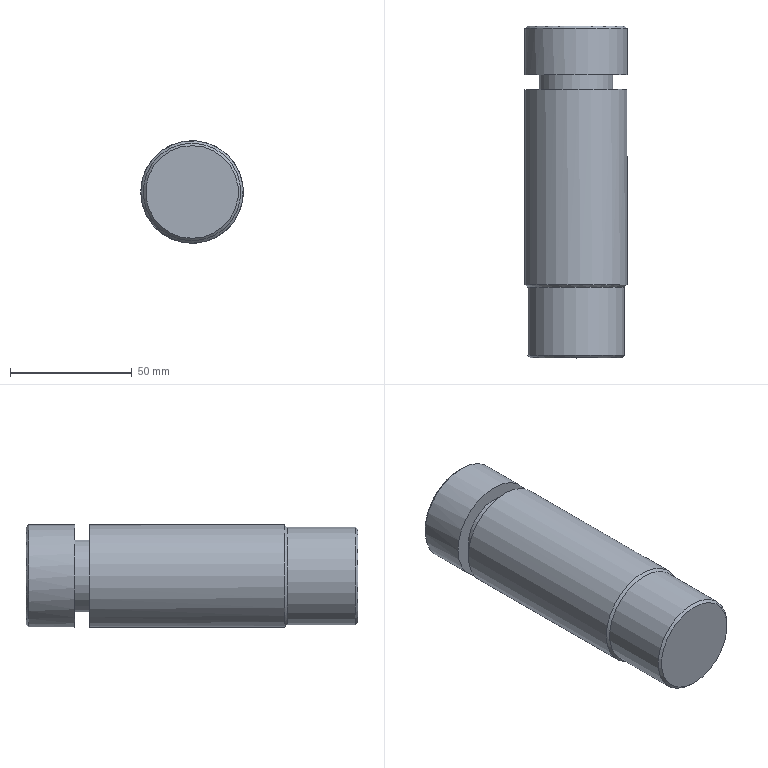Part | NX | features solid 2 | 1 solid | 11 faces | box 42 x 136 x 42 mm | volume 180422 mm3 | plane 4 | cylinder 4 | cone 3 | commonest cylinder face diameters 42 x2 30 x1 40 x1
STEP:
#1=CARTESIAN_POINT('',(1024.,425.,180.));
#2=VERTEX_POINT('',#1);
#3=CARTESIAN_POINT('',(1045.,425.,180.));
#4=DIRECTION('',(0.,1.,0.));
#5=DIRECTION('',(-1.,0.,0.));
#6=AXIS2_PLACEMENT_3D('',#3,#4,#5);
#7=CIRCLE('',#6,21.);
#8=EDGE_CURVE('',#2,#2,#7,.T.);
#9=ORIENTED_EDGE('',*,*,#8,.T.);
#10=EDGE_LOOP('',(#9));
#11=FACE_BOUND('',#10,.T.);
#12=CARTESIAN_POINT('',(1030.,425.,180.));
#13=VERTEX_POINT('',#12);
#14=CARTESIAN_POINT('',(1045.,425.,180.));
#15=DIRECTION('',(0.,1.,0.));
#16=DIRECTION('',(-1.,0.,0.));
#17=AXIS2_PLACEMENT_3D('',#14,#15,#16);
#18=CIRCLE('',#17,15.);
#19=EDGE_CURVE('',#13,#13,#18,.T.);
#20=ORIENTED_EDGE('',*,*,#19,.F.);
#21=EDGE_LOOP('',(#20));
#22=FACE_BOUND('',#21,.T.);
#23=CARTESIAN_POINT('',(1045.,425.,180.));
#24=DIRECTION('',(0.,1.,0.));
#25=DIRECTION('',(0.,0.,-1.));
#26=AXIS2_PLACEMENT_3D('',#23,#24,#25);
#27=PLANE('',#26);
#28=ADVANCED_FACE('',(#11,#22),#27,.T.);
#29=CARTESIAN_POINT('',(1024.,345.,180.));
#30=VERTEX_POINT('',#29);
#31=CARTESIAN_POINT('',(1045.,345.,180.));
#32=DIRECTION('',(0.,1.,0.));
#33=DIRECTION('',(-1.,0.,0.));
#34=AXIS2_PLACEMENT_3D('',#31,#32,#33);
#35=CIRCLE('',#34,21.);
#36=EDGE_CURVE('',#30,#30,#35,.T.);
#37=ORIENTED_EDGE('',*,*,#36,.T.);
#38=EDGE_LOOP('',(#37));
#39=FACE_BOUND('',#38,.T.);
#40=ORIENTED_EDGE('',*,*,#8,.F.);
#41=EDGE_LOOP('',(#40));
#42=FACE_BOUND('',#41,.T.);
#43=CARTESIAN_POINT('',(1045.,405.,180.));
#44=DIRECTION('',(0.,-1.,0.));
#45=DIRECTION('',(0.,0.,1.));
#46=AXIS2_PLACEMENT_3D('',#43,#44,#45);
#47=CYLINDRICAL_SURFACE('',#46,21.);
#48=ADVANCED_FACE('',(#39,#42),#47,.T.);
#49=CARTESIAN_POINT('',(1030.,431.,180.));
#50=VERTEX_POINT('',#49);
#51=CARTESIAN_POINT('',(1045.,431.,180.));
#52=DIRECTION('',(0.,1.,0.));
#53=DIRECTION('',(-1.,0.,0.));
#54=AXIS2_PLACEMENT_3D('',#51,#52,#53);
#55=CIRCLE('',#54,15.);
#56=EDGE_CURVE('',#50,#50,#55,.T.);
#57=ORIENTED_EDGE('',*,*,#56,.F.);
#58=EDGE_LOOP('',(#57));
#59=FACE_BOUND('',#58,.T.);
#60=ORIENTED_EDGE('',*,*,#19,.T.);
#61=EDGE_LOOP('',(#60));
#62=FACE_BOUND('',#61,.T.);
#63=CARTESIAN_POINT('',(1045.,431.,180.));
#64=DIRECTION('',(0.,-1.,0.));
#65=DIRECTION('',(0.,0.,1.));
#66=AXIS2_PLACEMENT_3D('',#63,#64,#65);
#67=CYLINDRICAL_SURFACE('',#66,15.);
#68=ADVANCED_FACE('',(#59,#62),#67,.T.);
#69=CARTESIAN_POINT('',(1024.,431.,180.));
#70=VERTEX_POINT('',#69);
#71=CARTESIAN_POINT('',(1045.,431.,180.));
#72=DIRECTION('',(0.,1.,0.));
#73=DIRECTION('',(-1.,0.,0.));
#74=AXIS2_PLACEMENT_3D('',#71,#72,#73);
#75=CIRCLE('',#74,21.);
#76=EDGE_CURVE('',#70,#70,#75,.T.);
#77=ORIENTED_EDGE('',*,*,#76,.F.);
#78=EDGE_LOOP('',(#77));
#79=FACE_BOUND('',#78,.T.);
#80=ORIENTED_EDGE('',*,*,#56,.T.);
#81=EDGE_LOOP('',(#80));
#82=FACE_BOUND('',#81,.T.);
#83=CARTESIAN_POINT('',(1045.,431.,180.));
#84=DIRECTION('',(0.,1.,0.));
#85=DIRECTION('',(0.,0.,-1.));
#86=AXIS2_PLACEMENT_3D('',#83,#84,#85);
#87=PLANE('',#86);
#88=ADVANCED_FACE('',(#79,#82),#87,.F.);
#89=CARTESIAN_POINT('',(1045.,450.,201.));
#90=VERTEX_POINT('',#89);
#91=CARTESIAN_POINT('',(1045.,450.,180.));
#92=DIRECTION('',(0.,1.,0.));
#93=DIRECTION('',(0.,0.,1.));
#94=AXIS2_PLACEMENT_3D('',#91,#92,#93);
#95=CIRCLE('',#94,21.);
#96=EDGE_CURVE('',#90,#90,#95,.F.);
#97=ORIENTED_EDGE('',*,*,#96,.T.);
#98=EDGE_LOOP('',(#97));
#99=FACE_BOUND('',#98,.T.);
#100=ORIENTED_EDGE('',*,*,#76,.T.);
#101=EDGE_LOOP('',(#100));
#102=FACE_BOUND('',#101,.T.);
#103=CARTESIAN_POINT('',(1045.,445.,180.));
#104=DIRECTION('',(0.,-1.,0.));
#105=DIRECTION('',(0.,0.,1.));
#106=AXIS2_PLACEMENT_3D('',#103,#104,#105);
#107=CYLINDRICAL_SURFACE('',#106,21.);
#108=ADVANCED_FACE('',(#99,#102),#107,.T.);
#109=CARTESIAN_POINT('',(1045.,344.,160.));
#110=VERTEX_POINT('',#109);
#111=CARTESIAN_POINT('',(1045.,344.,180.));
#112=DIRECTION('',(0.,1.,0.));
#113=DIRECTION('',(0.,0.,-1.));
#114=AXIS2_PLACEMENT_3D('',#111,#112,#113);
#115=CIRCLE('',#114,20.);
#116=EDGE_CURVE('',#110,#110,#115,.F.);
#117=ORIENTED_EDGE('',*,*,#116,.T.);
#118=EDGE_LOOP('',(#117));
#119=FACE_BOUND('',#118,.T.);
#120=CARTESIAN_POINT('',(1045.,316.,160.));
#121=VERTEX_POINT('',#120);
#122=CARTESIAN_POINT('',(1045.,316.,180.));
#123=DIRECTION('',(0.,1.,0.));
#124=DIRECTION('',(0.,0.,-1.));
#125=AXIS2_PLACEMENT_3D('',#122,#123,#124);
#126=CIRCLE('',#125,20.);
#127=EDGE_CURVE('',#121,#121,#126,.T.);
#128=ORIENTED_EDGE('',*,*,#127,.T.);
#129=EDGE_LOOP('',(#128));
#130=FACE_BOUND('',#129,.T.);
#131=CARTESIAN_POINT('',(1045.,275.,180.));
#132=DIRECTION('',(0.,1.,0.));
#133=DIRECTION('',(0.,0.,-1.));
#134=AXIS2_PLACEMENT_3D('',#131,#132,#133);
#135=CYLINDRICAL_SURFACE('',#134,20.);
#136=ADVANCED_FACE('',(#119,#130),#135,.T.);
#137=CARTESIAN_POINT('',(1045.,315.,161.));
#138=VERTEX_POINT('',#137);
#139=CARTESIAN_POINT('',(1045.,315.,180.));
#140=DIRECTION('',(0.,1.,0.));
#141=DIRECTION('',(0.,0.,-1.));
#142=AXIS2_PLACEMENT_3D('',#139,#140,#141);
#143=CIRCLE('',#142,19.);
#144=EDGE_CURVE('',#138,#138,#143,.F.);
#145=ORIENTED_EDGE('',*,*,#144,.T.);
#146=EDGE_LOOP('',(#145));
#147=FACE_BOUND('',#146,.T.);
#148=CARTESIAN_POINT('',(1045.,315.,180.));
#149=DIRECTION('',(0.,1.,0.));
#150=DIRECTION('',(0.,0.,-1.));
#151=AXIS2_PLACEMENT_3D('',#148,#149,#150);
#152=PLANE('',#151);
#153=ADVANCED_FACE('',(#147),#152,.F.);
#154=ORIENTED_EDGE('',*,*,#144,.F.);
#155=EDGE_LOOP('',(#154));
#156=FACE_BOUND('',#155,.T.);
#157=ORIENTED_EDGE('',*,*,#127,.F.);
#158=EDGE_LOOP('',(#157));
#159=FACE_BOUND('',#158,.T.);
#160=CARTESIAN_POINT('',(1045.,316.,180.));
#161=DIRECTION('',(0.,1.,0.));
#162=DIRECTION('',(0.,0.,-1.));
#163=AXIS2_PLACEMENT_3D('',#160,#161,#162);
#164=CONICAL_SURFACE('',#163,20.,0.7854);
#165=ADVANCED_FACE('',(#156,#159),#164,.T.);
#166=ORIENTED_EDGE('',*,*,#116,.F.);
#167=EDGE_LOOP('',(#166));
#168=FACE_BOUND('',#167,.T.);
#169=ORIENTED_EDGE('',*,*,#36,.F.);
#170=EDGE_LOOP('',(#169));
#171=FACE_BOUND('',#170,.T.);
#172=CARTESIAN_POINT('',(1045.,345.,180.));
#173=DIRECTION('',(0.,1.,0.));
#174=DIRECTION('',(0.,0.,-1.));
#175=AXIS2_PLACEMENT_3D('',#172,#173,#174);
#176=CONICAL_SURFACE('',#175,21.,0.7854);
#177=ADVANCED_FACE('',(#168,#171),#176,.T.);
#178=CARTESIAN_POINT('',(1045.,451.,200.));
#179=VERTEX_POINT('',#178);
#180=CARTESIAN_POINT('',(1045.,451.,180.));
#181=DIRECTION('',(0.,1.,0.));
#182=DIRECTION('',(0.,0.,1.));
#183=AXIS2_PLACEMENT_3D('',#180,#181,#182);
#184=CIRCLE('',#183,20.);
#185=EDGE_CURVE('',#179,#179,#184,.T.);
#186=ORIENTED_EDGE('',*,*,#185,.T.);
#187=EDGE_LOOP('',(#186));
#188=FACE_BOUND('',#187,.T.);
#189=CARTESIAN_POINT('',(1045.,451.,180.));
#190=DIRECTION('',(0.,1.,0.));
#191=DIRECTION('',(0.,0.,-1.));
#192=AXIS2_PLACEMENT_3D('',#189,#190,#191);
#193=PLANE('',#192);
#194=ADVANCED_FACE('',(#188),#193,.T.);
#195=ORIENTED_EDGE('',*,*,#96,.F.);
#196=EDGE_LOOP('',(#195));
#197=FACE_BOUND('',#196,.T.);
#198=ORIENTED_EDGE('',*,*,#185,.F.);
#199=EDGE_LOOP('',(#198));
#200=FACE_BOUND('',#199,.T.);
#201=CARTESIAN_POINT('',(1045.,451.,180.));
#202=DIRECTION('',(0.,-1.,0.));
#203=DIRECTION('',(0.,0.,-1.));
#204=AXIS2_PLACEMENT_3D('',#201,#202,#203);
#205=CONICAL_SURFACE('',#204,20.,0.7854);
#206=ADVANCED_FACE('',(#197,#200),#205,.T.);
#207=CLOSED_SHELL('',(#28,#48,#68,#88,#108,#136,#153,#165,#177,#194,#206));
#208=MANIFOLD_SOLID_BREP('',#207);
#209=(LENGTH_UNIT()NAMED_UNIT(*)SI_UNIT(.MILLI.,.METRE.));
#210=UNCERTAINTY_MEASURE_WITH_UNIT(LENGTH_MEASURE(0.00001),#209,'','');
#211=(NAMED_UNIT(*)PLANE_ANGLE_UNIT()SI_UNIT($,.RADIAN.));
#212=(NAMED_UNIT(*)SI_UNIT($,.STERADIAN.)SOLID_ANGLE_UNIT());
#213=(GEOMETRIC_REPRESENTATION_CONTEXT(3)GLOBAL_UNCERTAINTY_ASSIGNED_CONTEXT((#210))GLOBAL_UNIT_ASSIGNED_CONTEXT((#209,#211,#212))REPRESENTATION_CONTEXT('',''));
#214=ADVANCED_BREP_SHAPE_REPRESENTATION('',(#208),#213);